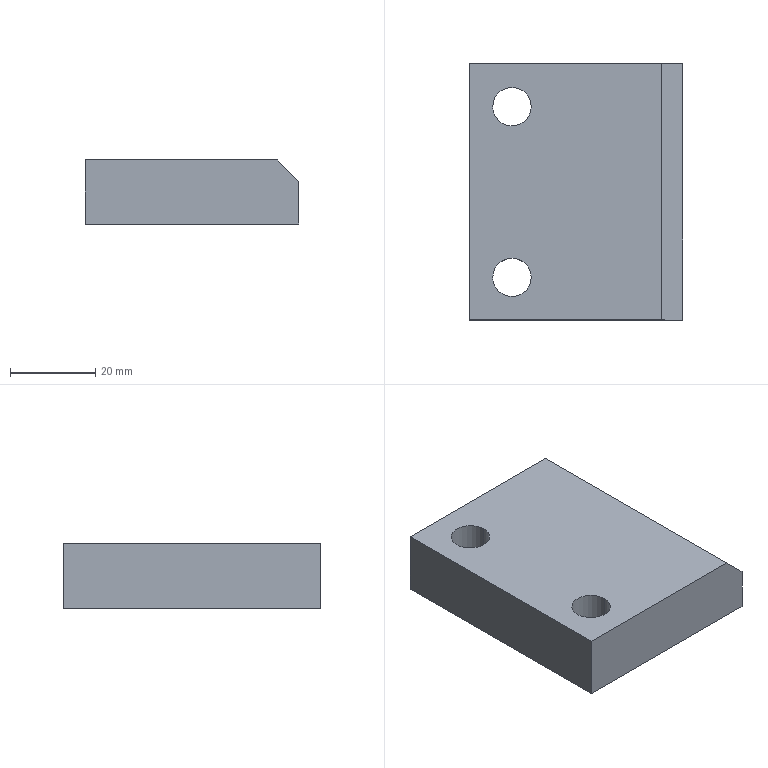Part | STEP file | Positioning_id1330_x_t | 1 solid | 11 faces | box 50 x 60 x 15 mm | volume 42341 mm3 | plane 7 | cylinder 4 | commonest cylinder face diameters 9 x4
STEP:
#1=CARTESIAN_POINT('',(0.,0.,0.));
#2=DIRECTION('',(0.,0.,1.));
#3=DIRECTION('',(1.,0.,0.));
#4=AXIS2_PLACEMENT_3D('',#1,#2,#3);
#5=CARTESIAN_POINT('',(-1027.502,770.,87.466));
#6=VERTEX_POINT('',#5);
#7=CARTESIAN_POINT('',(-1018.502,770.,87.466));
#8=VERTEX_POINT('',#7);
#9=CARTESIAN_POINT('',(-1023.002,770.,87.466));
#10=DIRECTION('',(0.,0.,-1.));
#11=DIRECTION('',(-1.,0.,0.));
#12=AXIS2_PLACEMENT_3D('',#9,#10,#11);
#13=CIRCLE('',#12,4.5);
#14=CARTESIAN_POINT('',(-1023.002,770.,72.466));
#15=DIRECTION('',(0.,0.,-1.));
#16=DIRECTION('',(-1.,0.,0.));
#17=AXIS2_PLACEMENT_3D('',#14,#15,#16);
#18=CYLINDRICAL_SURFACE('',#17,4.5);
#19=CARTESIAN_POINT('',(0.,-15.));
#20=DIRECTION('',(1.,0.));
#21=VECTOR('',#20,1.);
#22=LINE('',#19,#21);
#23=(GEOMETRIC_REPRESENTATION_CONTEXT(2)PARAMETRIC_REPRESENTATION_CONTEXT()REPRESENTATION_CONTEXT('',''));
#24=DEFINITIONAL_REPRESENTATION('',(#22),#23);
#25=PCURVE('',#18,#24);
#26=CARTESIAN_POINT('',(-1008.002,760.,87.466));
#27=DIRECTION('',(0.,0.,1.));
#28=DIRECTION('',(0.,1.,0.));
#29=AXIS2_PLACEMENT_3D('',#26,#27,#28);
#30=PLANE('',#29);
#31=CARTESIAN_POINT('',(10.,19.5));
#32=CARTESIAN_POINT('',(17.794,19.5));
#33=CARTESIAN_POINT('',(13.897,12.75));
#34=CARTESIAN_POINT('',(10.,6.));
#35=CARTESIAN_POINT('',(6.103,12.75));
#36=CARTESIAN_POINT('',(2.206,19.5));
#37=CARTESIAN_POINT('',(10.,19.5));
#38=(BOUNDED_CURVE()B_SPLINE_CURVE(2,(#31,#32,#33,#34,#35,#36,#37),.UNSPECIFIED.,.T.,.F.)B_SPLINE_CURVE_WITH_KNOTS((1,2,2,2,2,1),(-2.094,0.,2.094,4.189,6.283,8.378),.UNSPECIFIED.)CURVE()GEOMETRIC_REPRESENTATION_ITEM()RATIONAL_B_SPLINE_CURVE((1.,0.5,1.,0.5,1.,0.5,1.))REPRESENTATION_ITEM(''));
#39=(GEOMETRIC_REPRESENTATION_CONTEXT(2)PARAMETRIC_REPRESENTATION_CONTEXT()REPRESENTATION_CONTEXT('',''));
#40=DEFINITIONAL_REPRESENTATION('',(#38),#39);
#41=PCURVE('',#30,#40);
#42=SURFACE_CURVE('',#13,(#25,#41),.PCURVE_S1.);
#43=EDGE_CURVE('',#6,#8,#42,.T.);
#44=ORIENTED_EDGE('',*,*,#43,.T.);
#45=CARTESIAN_POINT('',(-1018.502,770.,72.466));
#46=VERTEX_POINT('',#45);
#47=CARTESIAN_POINT('',(-1018.502,770.,72.466));
#48=DIRECTION('',(0.,0.,-1.));
#49=VECTOR('',#48,1.);
#50=LINE('',#47,#49);
#51=CARTESIAN_POINT('',(3.142,0.));
#52=DIRECTION('',(0.,1.));
#53=VECTOR('',#52,1.);
#54=LINE('',#51,#53);
#55=(GEOMETRIC_REPRESENTATION_CONTEXT(2)PARAMETRIC_REPRESENTATION_CONTEXT()REPRESENTATION_CONTEXT('',''));
#56=DEFINITIONAL_REPRESENTATION('',(#54),#55);
#57=PCURVE('',#18,#56);
#58=CARTESIAN_POINT('',(-1023.002,770.,72.466));
#59=DIRECTION('',(0.,0.,-1.));
#60=DIRECTION('',(-1.,0.,0.));
#61=AXIS2_PLACEMENT_3D('',#58,#59,#60);
#62=CYLINDRICAL_SURFACE('',#61,4.5);
#63=CARTESIAN_POINT('',(3.142,0.));
#64=DIRECTION('',(0.,1.));
#65=VECTOR('',#64,1.);
#66=LINE('',#63,#65);
#67=(GEOMETRIC_REPRESENTATION_CONTEXT(2)PARAMETRIC_REPRESENTATION_CONTEXT()REPRESENTATION_CONTEXT('',''));
#68=DEFINITIONAL_REPRESENTATION('',(#66),#67);
#69=PCURVE('',#62,#68);
#70=SURFACE_CURVE('',#50,(#57,#69),.PCURVE_S1.);
#71=EDGE_CURVE('',#8,#46,#70,.T.);
#72=ORIENTED_EDGE('',*,*,#71,.T.);
#73=CARTESIAN_POINT('',(-1027.502,770.,72.466));
#74=VERTEX_POINT('',#73);
#75=CARTESIAN_POINT('',(-1023.002,770.,72.466));
#76=DIRECTION('',(0.,0.,-1.));
#77=DIRECTION('',(-1.,0.,0.));
#78=AXIS2_PLACEMENT_3D('',#75,#76,#77);
#79=CIRCLE('',#78,4.5);
#80=CARTESIAN_POINT('',(0.,0.));
#81=DIRECTION('',(1.,0.));
#82=VECTOR('',#81,1.);
#83=LINE('',#80,#82);
#84=(GEOMETRIC_REPRESENTATION_CONTEXT(2)PARAMETRIC_REPRESENTATION_CONTEXT()REPRESENTATION_CONTEXT('',''));
#85=DEFINITIONAL_REPRESENTATION('',(#83),#84);
#86=PCURVE('',#18,#85);
#87=CARTESIAN_POINT('',(-1008.002,760.,72.466));
#88=DIRECTION('',(0.,0.,-1.));
#89=DIRECTION('',(0.,-1.,0.));
#90=AXIS2_PLACEMENT_3D('',#87,#88,#89);
#91=PLANE('',#90);
#92=CARTESIAN_POINT('',(-10.,15.));
#93=DIRECTION('',(0.,1.));
#94=AXIS2_PLACEMENT_2D('',#92,#93);
#95=CIRCLE('',#94,4.5);
#96=(GEOMETRIC_REPRESENTATION_CONTEXT(2)PARAMETRIC_REPRESENTATION_CONTEXT()REPRESENTATION_CONTEXT('',''));
#97=DEFINITIONAL_REPRESENTATION('',(#95),#96);
#98=PCURVE('',#91,#97);
#99=SURFACE_CURVE('',#79,(#86,#98),.PCURVE_S1.);
#100=EDGE_CURVE('',#74,#46,#99,.T.);
#101=ORIENTED_EDGE('',*,*,#100,.F.);
#102=CARTESIAN_POINT('',(-1027.502,770.,72.466));
#103=DIRECTION('',(0.,0.,1.));
#104=VECTOR('',#103,1.);
#105=LINE('',#102,#104);
#106=CARTESIAN_POINT('',(0.,0.));
#107=DIRECTION('',(0.,-1.));
#108=VECTOR('',#107,1.);
#109=LINE('',#106,#108);
#110=(GEOMETRIC_REPRESENTATION_CONTEXT(2)PARAMETRIC_REPRESENTATION_CONTEXT()REPRESENTATION_CONTEXT('',''));
#111=DEFINITIONAL_REPRESENTATION('',(#109),#110);
#112=PCURVE('',#18,#111);
#113=CARTESIAN_POINT('',(6.283,0.));
#114=DIRECTION('',(0.,-1.));
#115=VECTOR('',#114,1.);
#116=LINE('',#113,#115);
#117=(GEOMETRIC_REPRESENTATION_CONTEXT(2)PARAMETRIC_REPRESENTATION_CONTEXT()REPRESENTATION_CONTEXT('',''));
#118=DEFINITIONAL_REPRESENTATION('',(#116),#117);
#119=PCURVE('',#62,#118);
#120=SURFACE_CURVE('',#105,(#112,#119),.PCURVE_S1.);
#121=EDGE_CURVE('',#74,#6,#120,.T.);
#122=ORIENTED_EDGE('',*,*,#121,.T.);
#123=EDGE_LOOP('',(#44,#72,#101,#122));
#124=FACE_BOUND('',#123,.F.);
#125=ADVANCED_FACE('',(#124),#18,.F.);
#126=CARTESIAN_POINT('',(-1027.502,810.,87.466));
#127=VERTEX_POINT('',#126);
#128=CARTESIAN_POINT('',(-1018.502,810.,87.466));
#129=VERTEX_POINT('',#128);
#130=CARTESIAN_POINT('',(-1023.002,810.,87.466));
#131=DIRECTION('',(0.,0.,-1.));
#132=DIRECTION('',(-1.,0.,0.));
#133=AXIS2_PLACEMENT_3D('',#130,#131,#132);
#134=CIRCLE('',#133,4.5);
#135=CARTESIAN_POINT('',(-1023.002,810.,72.466));
#136=DIRECTION('',(0.,0.,-1.));
#137=DIRECTION('',(-1.,0.,0.));
#138=AXIS2_PLACEMENT_3D('',#135,#136,#137);
#139=CYLINDRICAL_SURFACE('',#138,4.5);
#140=CARTESIAN_POINT('',(0.,-15.));
#141=DIRECTION('',(1.,0.));
#142=VECTOR('',#141,1.);
#143=LINE('',#140,#142);
#144=(GEOMETRIC_REPRESENTATION_CONTEXT(2)PARAMETRIC_REPRESENTATION_CONTEXT()REPRESENTATION_CONTEXT('',''));
#145=DEFINITIONAL_REPRESENTATION('',(#143),#144);
#146=PCURVE('',#139,#145);
#147=CARTESIAN_POINT('',(50.,19.5));
#148=CARTESIAN_POINT('',(57.794,19.5));
#149=CARTESIAN_POINT('',(53.897,12.75));
#150=CARTESIAN_POINT('',(50.,6.));
#151=CARTESIAN_POINT('',(46.103,12.75));
#152=CARTESIAN_POINT('',(42.206,19.5));
#153=CARTESIAN_POINT('',(50.,19.5));
#154=(BOUNDED_CURVE()B_SPLINE_CURVE(2,(#147,#148,#149,#150,#151,#152,#153),.UNSPECIFIED.,.T.,.F.)B_SPLINE_CURVE_WITH_KNOTS((1,2,2,2,2,1),(-2.094,0.,2.094,4.189,6.283,8.378),.UNSPECIFIED.)CURVE()GEOMETRIC_REPRESENTATION_ITEM()RATIONAL_B_SPLINE_CURVE((1.,0.5,1.,0.5,1.,0.5,1.))REPRESENTATION_ITEM(''));
#155=(GEOMETRIC_REPRESENTATION_CONTEXT(2)PARAMETRIC_REPRESENTATION_CONTEXT()REPRESENTATION_CONTEXT('',''));
#156=DEFINITIONAL_REPRESENTATION('',(#154),#155);
#157=PCURVE('',#30,#156);
#158=SURFACE_CURVE('',#134,(#146,#157),.PCURVE_S1.);
#159=EDGE_CURVE('',#127,#129,#158,.T.);
#160=ORIENTED_EDGE('',*,*,#159,.T.);
#161=CARTESIAN_POINT('',(-1018.502,810.,72.466));
#162=VERTEX_POINT('',#161);
#163=CARTESIAN_POINT('',(-1018.502,810.,72.466));
#164=DIRECTION('',(0.,0.,-1.));
#165=VECTOR('',#164,1.);
#166=LINE('',#163,#165);
#167=CARTESIAN_POINT('',(3.142,0.));
#168=DIRECTION('',(0.,1.));
#169=VECTOR('',#168,1.);
#170=LINE('',#167,#169);
#171=(GEOMETRIC_REPRESENTATION_CONTEXT(2)PARAMETRIC_REPRESENTATION_CONTEXT()REPRESENTATION_CONTEXT('',''));
#172=DEFINITIONAL_REPRESENTATION('',(#170),#171);
#173=PCURVE('',#139,#172);
#174=CARTESIAN_POINT('',(-1023.002,810.,72.466));
#175=DIRECTION('',(0.,0.,-1.));
#176=DIRECTION('',(-1.,0.,0.));
#177=AXIS2_PLACEMENT_3D('',#174,#175,#176);
#178=CYLINDRICAL_SURFACE('',#177,4.5);
#179=CARTESIAN_POINT('',(3.142,0.));
#180=DIRECTION('',(0.,1.));
#181=VECTOR('',#180,1.);
#182=LINE('',#179,#181);
#183=(GEOMETRIC_REPRESENTATION_CONTEXT(2)PARAMETRIC_REPRESENTATION_CONTEXT()REPRESENTATION_CONTEXT('',''));
#184=DEFINITIONAL_REPRESENTATION('',(#182),#183);
#185=PCURVE('',#178,#184);
#186=SURFACE_CURVE('',#166,(#173,#185),.PCURVE_S1.);
#187=EDGE_CURVE('',#129,#162,#186,.T.);
#188=ORIENTED_EDGE('',*,*,#187,.T.);
#189=CARTESIAN_POINT('',(-1027.502,810.,72.466));
#190=VERTEX_POINT('',#189);
#191=CARTESIAN_POINT('',(-1023.002,810.,72.466));
#192=DIRECTION('',(0.,0.,-1.));
#193=DIRECTION('',(-1.,0.,0.));
#194=AXIS2_PLACEMENT_3D('',#191,#192,#193);
#195=CIRCLE('',#194,4.5);
#196=CARTESIAN_POINT('',(0.,0.));
#197=DIRECTION('',(1.,0.));
#198=VECTOR('',#197,1.);
#199=LINE('',#196,#198);
#200=(GEOMETRIC_REPRESENTATION_CONTEXT(2)PARAMETRIC_REPRESENTATION_CONTEXT()REPRESENTATION_CONTEXT('',''));
#201=DEFINITIONAL_REPRESENTATION('',(#199),#200);
#202=PCURVE('',#139,#201);
#203=CARTESIAN_POINT('',(-50.,15.));
#204=DIRECTION('',(0.,1.));
#205=AXIS2_PLACEMENT_2D('',#203,#204);
#206=CIRCLE('',#205,4.5);
#207=(GEOMETRIC_REPRESENTATION_CONTEXT(2)PARAMETRIC_REPRESENTATION_CONTEXT()REPRESENTATION_CONTEXT('',''));
#208=DEFINITIONAL_REPRESENTATION('',(#206),#207);
#209=PCURVE('',#91,#208);
#210=SURFACE_CURVE('',#195,(#202,#209),.PCURVE_S1.);
#211=EDGE_CURVE('',#190,#162,#210,.T.);
#212=ORIENTED_EDGE('',*,*,#211,.F.);
#213=CARTESIAN_POINT('',(-1027.502,810.,72.466));
#214=DIRECTION('',(0.,0.,1.));
#215=VECTOR('',#214,1.);
#216=LINE('',#213,#215);
#217=CARTESIAN_POINT('',(0.,0.));
#218=DIRECTION('',(0.,-1.));
#219=VECTOR('',#218,1.);
#220=LINE('',#217,#219);
#221=(GEOMETRIC_REPRESENTATION_CONTEXT(2)PARAMETRIC_REPRESENTATION_CONTEXT()REPRESENTATION_CONTEXT('',''));
#222=DEFINITIONAL_REPRESENTATION('',(#220),#221);
#223=PCURVE('',#139,#222);
#224=CARTESIAN_POINT('',(6.283,0.));
#225=DIRECTION('',(0.,-1.));
#226=VECTOR('',#225,1.);
#227=LINE('',#224,#226);
#228=(GEOMETRIC_REPRESENTATION_CONTEXT(2)PARAMETRIC_REPRESENTATION_CONTEXT()REPRESENTATION_CONTEXT('',''));
#229=DEFINITIONAL_REPRESENTATION('',(#227),#228);
#230=PCURVE('',#178,#229);
#231=SURFACE_CURVE('',#216,(#223,#230),.PCURVE_S1.);
#232=EDGE_CURVE('',#190,#127,#231,.T.);
#233=ORIENTED_EDGE('',*,*,#232,.T.);
#234=EDGE_LOOP('',(#160,#188,#212,#233));
#235=FACE_BOUND('',#234,.F.);
#236=ADVANCED_FACE('',(#235),#139,.F.);
#237=CARTESIAN_POINT('',(-988.002,760.,87.466));
#238=VERTEX_POINT('',#237);
#239=CARTESIAN_POINT('',(-983.002,760.,82.466));
#240=VERTEX_POINT('',#239);
#241=CARTESIAN_POINT('',(-988.002,760.,87.466));
#242=DIRECTION('',(0.7071,0.,-0.7071));
#243=VECTOR('',#242,1.);
#244=LINE('',#241,#243);
#245=CARTESIAN_POINT('',(-983.002,760.,82.466));
#246=DIRECTION('',(-0.7071,0.,-0.7071));
#247=DIRECTION('',(0.7071,0.,-0.7071));
#248=AXIS2_PLACEMENT_3D('',#245,#246,#247);
#249=PLANE('',#248);
#250=CARTESIAN_POINT('',(-7.071,0.));
#251=DIRECTION('',(1.,0.));
#252=VECTOR('',#251,1.);
#253=LINE('',#250,#252);
#254=(GEOMETRIC_REPRESENTATION_CONTEXT(2)PARAMETRIC_REPRESENTATION_CONTEXT()REPRESENTATION_CONTEXT('',''));
#255=DEFINITIONAL_REPRESENTATION('',(#253),#254);
#256=PCURVE('',#249,#255);
#257=CARTESIAN_POINT('',(-1008.002,760.,79.966));
#258=DIRECTION('',(0.,-1.,0.));
#259=DIRECTION('',(0.,0.,1.));
#260=AXIS2_PLACEMENT_3D('',#257,#258,#259);
#261=PLANE('',#260);
#262=CARTESIAN_POINT('',(7.5,-20.));
#263=DIRECTION('',(-0.7071,-0.7071));
#264=VECTOR('',#263,1.);
#265=LINE('',#262,#264);
#266=(GEOMETRIC_REPRESENTATION_CONTEXT(2)PARAMETRIC_REPRESENTATION_CONTEXT()REPRESENTATION_CONTEXT('',''));
#267=DEFINITIONAL_REPRESENTATION('',(#265),#266);
#268=PCURVE('',#261,#267);
#269=SURFACE_CURVE('',#244,(#256,#268),.PCURVE_S1.);
#270=EDGE_CURVE('',#238,#240,#269,.T.);
#271=ORIENTED_EDGE('',*,*,#270,.T.);
#272=CARTESIAN_POINT('',(-983.002,820.,82.466));
#273=VERTEX_POINT('',#272);
#274=CARTESIAN_POINT('',(-983.002,760.,82.466));
#275=DIRECTION('',(0.,1.,0.));
#276=VECTOR('',#275,1.);
#277=LINE('',#274,#276);
#278=CARTESIAN_POINT('',(0.,0.));
#279=DIRECTION('',(0.,-1.));
#280=VECTOR('',#279,1.);
#281=LINE('',#278,#280);
#282=(GEOMETRIC_REPRESENTATION_CONTEXT(2)PARAMETRIC_REPRESENTATION_CONTEXT()REPRESENTATION_CONTEXT('',''));
#283=DEFINITIONAL_REPRESENTATION('',(#281),#282);
#284=PCURVE('',#249,#283);
#285=CARTESIAN_POINT('',(-983.002,760.,79.966));
#286=DIRECTION('',(1.,0.,0.));
#287=DIRECTION('',(0.,1.,0.));
#288=AXIS2_PLACEMENT_3D('',#285,#286,#287);
#289=PLANE('',#288);
#290=CARTESIAN_POINT('',(0.,2.5));
#291=DIRECTION('',(1.,0.));
#292=VECTOR('',#291,1.);
#293=LINE('',#290,#292);
#294=(GEOMETRIC_REPRESENTATION_CONTEXT(2)PARAMETRIC_REPRESENTATION_CONTEXT()REPRESENTATION_CONTEXT('',''));
#295=DEFINITIONAL_REPRESENTATION('',(#293),#294);
#296=PCURVE('',#289,#295);
#297=SURFACE_CURVE('',#277,(#284,#296),.PCURVE_S1.);
#298=EDGE_CURVE('',#240,#273,#297,.T.);
#299=ORIENTED_EDGE('',*,*,#298,.T.);
#300=CARTESIAN_POINT('',(-988.002,820.,87.466));
#301=VERTEX_POINT('',#300);
#302=CARTESIAN_POINT('',(-983.002,820.,82.466));
#303=DIRECTION('',(-0.7071,0.,0.7071));
#304=VECTOR('',#303,1.);
#305=LINE('',#302,#304);
#306=CARTESIAN_POINT('',(0.,-60.));
#307=DIRECTION('',(-1.,0.));
#308=VECTOR('',#307,1.);
#309=LINE('',#306,#308);
#310=(GEOMETRIC_REPRESENTATION_CONTEXT(2)PARAMETRIC_REPRESENTATION_CONTEXT()REPRESENTATION_CONTEXT('',''));
#311=DEFINITIONAL_REPRESENTATION('',(#309),#310);
#312=PCURVE('',#249,#311);
#313=CARTESIAN_POINT('',(-1008.002,820.,79.966));
#314=DIRECTION('',(0.,1.,0.));
#315=DIRECTION('',(0.,0.,-1.));
#316=AXIS2_PLACEMENT_3D('',#313,#314,#315);
#317=PLANE('',#316);
#318=CARTESIAN_POINT('',(-2.5,-25.));
#319=DIRECTION('',(-0.7071,0.7071));
#320=VECTOR('',#319,1.);
#321=LINE('',#318,#320);
#322=(GEOMETRIC_REPRESENTATION_CONTEXT(2)PARAMETRIC_REPRESENTATION_CONTEXT()REPRESENTATION_CONTEXT('',''));
#323=DEFINITIONAL_REPRESENTATION('',(#321),#322);
#324=PCURVE('',#317,#323);
#325=SURFACE_CURVE('',#305,(#312,#324),.PCURVE_S1.);
#326=EDGE_CURVE('',#273,#301,#325,.T.);
#327=ORIENTED_EDGE('',*,*,#326,.T.);
#328=CARTESIAN_POINT('',(-988.002,820.,87.466));
#329=DIRECTION('',(0.,-1.,0.));
#330=VECTOR('',#329,1.);
#331=LINE('',#328,#330);
#332=CARTESIAN_POINT('',(-7.071,-60.));
#333=DIRECTION('',(0.,1.));
#334=VECTOR('',#333,1.);
#335=LINE('',#332,#334);
#336=(GEOMETRIC_REPRESENTATION_CONTEXT(2)PARAMETRIC_REPRESENTATION_CONTEXT()REPRESENTATION_CONTEXT('',''));
#337=DEFINITIONAL_REPRESENTATION('',(#335),#336);
#338=PCURVE('',#249,#337);
#339=CARTESIAN_POINT('',(60.,-20.));
#340=DIRECTION('',(-1.,0.));
#341=VECTOR('',#340,1.);
#342=LINE('',#339,#341);
#343=(GEOMETRIC_REPRESENTATION_CONTEXT(2)PARAMETRIC_REPRESENTATION_CONTEXT()REPRESENTATION_CONTEXT('',''));
#344=DEFINITIONAL_REPRESENTATION('',(#342),#343);
#345=PCURVE('',#30,#344);
#346=SURFACE_CURVE('',#331,(#338,#345),.PCURVE_S1.);
#347=EDGE_CURVE('',#301,#238,#346,.T.);
#348=ORIENTED_EDGE('',*,*,#347,.T.);
#349=EDGE_LOOP('',(#271,#299,#327,#348));
#350=FACE_BOUND('',#349,.T.);
#351=ADVANCED_FACE('',(#350),#249,.F.);
#352=CARTESIAN_POINT('',(-1018.502,810.,87.466));
#353=CARTESIAN_POINT('',(-1018.502,805.5,87.466));
#354=CARTESIAN_POINT('',(-1023.002,803.25,87.466));
#355=CARTESIAN_POINT('',(-1027.502,805.5,87.466));
#356=CARTESIAN_POINT('',(-1027.502,810.,87.466));
#357=(BOUNDED_CURVE()B_SPLINE_CURVE(4,(#352,#353,#354,#355,#356),.UNSPECIFIED.,.F.,.F.)B_SPLINE_CURVE_WITH_KNOTS((5,5),(0.,1.),.PIECEWISE_BEZIER_KNOTS.)CURVE()GEOMETRIC_REPRESENTATION_ITEM()RATIONAL_B_SPLINE_CURVE((1.,0.7071,0.6667,0.7071,1.))REPRESENTATION_ITEM(''));
#358=CARTESIAN_POINT('',(50.,10.5));
#359=CARTESIAN_POINT('',(45.5,10.5));
#360=CARTESIAN_POINT('',(43.25,15.));
#361=CARTESIAN_POINT('',(45.5,19.5));
#362=CARTESIAN_POINT('',(50.,19.5));
#363=(BOUNDED_CURVE()B_SPLINE_CURVE(4,(#358,#359,#360,#361,#362),.UNSPECIFIED.,.F.,.F.)B_SPLINE_CURVE_WITH_KNOTS((5,5),(0.,1.),.PIECEWISE_BEZIER_KNOTS.)CURVE()GEOMETRIC_REPRESENTATION_ITEM()RATIONAL_B_SPLINE_CURVE((1.,0.7071,0.6667,0.7071,1.))REPRESENTATION_ITEM(''));
#364=(GEOMETRIC_REPRESENTATION_CONTEXT(2)PARAMETRIC_REPRESENTATION_CONTEXT()REPRESENTATION_CONTEXT('',''));
#365=DEFINITIONAL_REPRESENTATION('',(#363),#364);
#366=PCURVE('',#30,#365);
#367=CARTESIAN_POINT('',(3.142,-15.));
#368=CARTESIAN_POINT('',(3.184,-15.));
#369=CARTESIAN_POINT('',(3.271,-15.));
#370=CARTESIAN_POINT('',(3.405,-15.));
#371=CARTESIAN_POINT('',(3.542,-15.));
#372=CARTESIAN_POINT('',(3.681,-15.));
#373=CARTESIAN_POINT('',(3.823,-15.));
#374=CARTESIAN_POINT('',(3.968,-15.));
#375=CARTESIAN_POINT('',(4.114,-15.));
#376=CARTESIAN_POINT('',(4.262,-15.));
#377=CARTESIAN_POINT('',(4.412,-15.));
#378=CARTESIAN_POINT('',(4.562,-15.));
#379=CARTESIAN_POINT('',(4.712,-15.));
#380=CARTESIAN_POINT('',(4.863,-15.));
#381=CARTESIAN_POINT('',(5.013,-15.));
#382=CARTESIAN_POINT('',(5.163,-15.));
#383=CARTESIAN_POINT('',(5.311,-15.));
#384=CARTESIAN_POINT('',(5.457,-15.));
#385=CARTESIAN_POINT('',(5.602,-15.));
#386=CARTESIAN_POINT('',(5.744,-15.));
#387=CARTESIAN_POINT('',(5.883,-15.));
#388=CARTESIAN_POINT('',(6.02,-15.));
#389=CARTESIAN_POINT('',(6.153,-15.));
#390=CARTESIAN_POINT('',(6.24,-15.));
#391=CARTESIAN_POINT('',(6.283,-15.));
#392=B_SPLINE_CURVE_WITH_KNOTS('',3,(#367,#368,#369,#370,#371,#372,#373,#374,#375,#376,#377,#378,#379,#380,#381,#382,#383,#384,#385,#386,#387,#388,#389,#390,#391),.UNSPECIFIED.,.F.,.F.,(4,1,1,1,1,1,1,1,1,1,1,1,1,1,1,1,1,1,1,1,1,1,4),(0.,0.04545,0.09091,0.1364,0.1818,0.2273,0.2727,0.3182,0.3636,0.4091,0.4545,0.5,0.5455,0.5909,0.6364,0.6818,0.7273,0.7727,0.8182,0.8636,0.9091,0.9545,1.),.QUASI_UNIFORM_KNOTS.);
#393=(GEOMETRIC_REPRESENTATION_CONTEXT(2)PARAMETRIC_REPRESENTATION_CONTEXT()REPRESENTATION_CONTEXT('',''));
#394=DEFINITIONAL_REPRESENTATION('',(#392),#393);
#395=PCURVE('',#178,#394);
#396=SURFACE_CURVE('',#357,(#366,#395),.PCURVE_S1.);
#397=EDGE_CURVE('',#129,#127,#396,.T.);
#398=ORIENTED_EDGE('',*,*,#397,.T.);
#399=ORIENTED_EDGE('',*,*,#159,.T.);
#400=EDGE_LOOP('',(#398,#399));
#401=FACE_BOUND('',#400,.T.);
#402=CARTESIAN_POINT('',(-1018.502,770.,87.466));
#403=CARTESIAN_POINT('',(-1018.502,765.5,87.466));
#404=CARTESIAN_POINT('',(-1023.002,763.25,87.466));
#405=CARTESIAN_POINT('',(-1027.502,765.5,87.466));
#406=CARTESIAN_POINT('',(-1027.502,770.,87.466));
#407=(BOUNDED_CURVE()B_SPLINE_CURVE(4,(#402,#403,#404,#405,#406),.UNSPECIFIED.,.F.,.F.)B_SPLINE_CURVE_WITH_KNOTS((5,5),(0.,1.),.PIECEWISE_BEZIER_KNOTS.)CURVE()GEOMETRIC_REPRESENTATION_ITEM()RATIONAL_B_SPLINE_CURVE((1.,0.7071,0.6667,0.7071,1.))REPRESENTATION_ITEM(''));
#408=CARTESIAN_POINT('',(10.,10.5));
#409=CARTESIAN_POINT('',(5.5,10.5));
#410=CARTESIAN_POINT('',(3.25,15.));
#411=CARTESIAN_POINT('',(5.5,19.5));
#412=CARTESIAN_POINT('',(10.,19.5));
#413=(BOUNDED_CURVE()B_SPLINE_CURVE(4,(#408,#409,#410,#411,#412),.UNSPECIFIED.,.F.,.F.)B_SPLINE_CURVE_WITH_KNOTS((5,5),(0.,1.),.PIECEWISE_BEZIER_KNOTS.)CURVE()GEOMETRIC_REPRESENTATION_ITEM()RATIONAL_B_SPLINE_CURVE((1.,0.7071,0.6667,0.7071,1.))REPRESENTATION_ITEM(''));
#414=(GEOMETRIC_REPRESENTATION_CONTEXT(2)PARAMETRIC_REPRESENTATION_CONTEXT()REPRESENTATION_CONTEXT('',''));
#415=DEFINITIONAL_REPRESENTATION('',(#413),#414);
#416=PCURVE('',#30,#415);
#417=CARTESIAN_POINT('',(3.142,-15.));
#418=CARTESIAN_POINT('',(3.184,-15.));
#419=CARTESIAN_POINT('',(3.271,-15.));
#420=CARTESIAN_POINT('',(3.405,-15.));
#421=CARTESIAN_POINT('',(3.542,-15.));
#422=CARTESIAN_POINT('',(3.681,-15.));
#423=CARTESIAN_POINT('',(3.823,-15.));
#424=CARTESIAN_POINT('',(3.968,-15.));
#425=CARTESIAN_POINT('',(4.114,-15.));
#426=CARTESIAN_POINT('',(4.262,-15.));
#427=CARTESIAN_POINT('',(4.412,-15.));
#428=CARTESIAN_POINT('',(4.562,-15.));
#429=CARTESIAN_POINT('',(4.712,-15.));
#430=CARTESIAN_POINT('',(4.863,-15.));
#431=CARTESIAN_POINT('',(5.013,-15.));
#432=CARTESIAN_POINT('',(5.163,-15.));
#433=CARTESIAN_POINT('',(5.311,-15.));
#434=CARTESIAN_POINT('',(5.457,-15.));
#435=CARTESIAN_POINT('',(5.602,-15.));
#436=CARTESIAN_POINT('',(5.744,-15.));
#437=CARTESIAN_POINT('',(5.883,-15.));
#438=CARTESIAN_POINT('',(6.02,-15.));
#439=CARTESIAN_POINT('',(6.153,-15.));
#440=CARTESIAN_POINT('',(6.24,-15.));
#441=CARTESIAN_POINT('',(6.283,-15.));
#442=B_SPLINE_CURVE_WITH_KNOTS('',3,(#417,#418,#419,#420,#421,#422,#423,#424,#425,#426,#427,#428,#429,#430,#431,#432,#433,#434,#435,#436,#437,#438,#439,#440,#441),.UNSPECIFIED.,.F.,.F.,(4,1,1,1,1,1,1,1,1,1,1,1,1,1,1,1,1,1,1,1,1,1,4),(0.,0.04545,0.09091,0.1364,0.1818,0.2273,0.2727,0.3182,0.3636,0.4091,0.4545,0.5,0.5455,0.5909,0.6364,0.6818,0.7273,0.7727,0.8182,0.8636,0.9091,0.9545,1.),.QUASI_UNIFORM_KNOTS.);
#443=(GEOMETRIC_REPRESENTATION_CONTEXT(2)PARAMETRIC_REPRESENTATION_CONTEXT()REPRESENTATION_CONTEXT('',''));
#444=DEFINITIONAL_REPRESENTATION('',(#442),#443);
#445=PCURVE('',#62,#444);
#446=SURFACE_CURVE('',#407,(#416,#445),.PCURVE_S1.);
#447=EDGE_CURVE('',#8,#6,#446,.T.);
#448=ORIENTED_EDGE('',*,*,#447,.T.);
#449=ORIENTED_EDGE('',*,*,#43,.T.);
#450=EDGE_LOOP('',(#448,#449));
#451=FACE_BOUND('',#450,.T.);
#452=CARTESIAN_POINT('',(-1033.002,820.,87.466));
#453=VERTEX_POINT('',#452);
#454=CARTESIAN_POINT('',(-1033.002,820.,87.466));
#455=DIRECTION('',(1.,0.,0.));
#456=VECTOR('',#455,1.);
#457=LINE('',#454,#456);
#458=CARTESIAN_POINT('',(60.,25.));
#459=DIRECTION('',(0.,-1.));
#460=VECTOR('',#459,1.);
#461=LINE('',#458,#460);
#462=(GEOMETRIC_REPRESENTATION_CONTEXT(2)PARAMETRIC_REPRESENTATION_CONTEXT()REPRESENTATION_CONTEXT('',''));
#463=DEFINITIONAL_REPRESENTATION('',(#461),#462);
#464=PCURVE('',#30,#463);
#465=CARTESIAN_POINT('',(-7.5,25.));
#466=DIRECTION('',(0.,-1.));
#467=VECTOR('',#466,1.);
#468=LINE('',#465,#467);
#469=(GEOMETRIC_REPRESENTATION_CONTEXT(2)PARAMETRIC_REPRESENTATION_CONTEXT()REPRESENTATION_CONTEXT('',''));
#470=DEFINITIONAL_REPRESENTATION('',(#468),#469);
#471=PCURVE('',#317,#470);
#472=SURFACE_CURVE('',#457,(#464,#471),.PCURVE_S1.);
#473=EDGE_CURVE('',#453,#301,#472,.T.);
#474=ORIENTED_EDGE('',*,*,#473,.F.);
#475=CARTESIAN_POINT('',(-1033.002,760.,87.466));
#476=VERTEX_POINT('',#475);
#477=CARTESIAN_POINT('',(-1033.002,760.,87.466));
#478=DIRECTION('',(0.,1.,0.));
#479=VECTOR('',#478,1.);
#480=LINE('',#477,#479);
#481=CARTESIAN_POINT('',(0.,25.));
#482=DIRECTION('',(1.,0.));
#483=VECTOR('',#482,1.);
#484=LINE('',#481,#483);
#485=(GEOMETRIC_REPRESENTATION_CONTEXT(2)PARAMETRIC_REPRESENTATION_CONTEXT()REPRESENTATION_CONTEXT('',''));
#486=DEFINITIONAL_REPRESENTATION('',(#484),#485);
#487=PCURVE('',#30,#486);
#488=CARTESIAN_POINT('',(-1033.002,760.,79.966));
#489=DIRECTION('',(-1.,0.,0.));
#490=DIRECTION('',(0.,-1.,0.));
#491=AXIS2_PLACEMENT_3D('',#488,#489,#490);
#492=PLANE('',#491);
#493=CARTESIAN_POINT('',(0.,7.5));
#494=DIRECTION('',(-1.,0.));
#495=VECTOR('',#494,1.);
#496=LINE('',#493,#495);
#497=(GEOMETRIC_REPRESENTATION_CONTEXT(2)PARAMETRIC_REPRESENTATION_CONTEXT()REPRESENTATION_CONTEXT('',''));
#498=DEFINITIONAL_REPRESENTATION('',(#496),#497);
#499=PCURVE('',#492,#498);
#500=SURFACE_CURVE('',#480,(#487,#499),.PCURVE_S1.);
#501=EDGE_CURVE('',#476,#453,#500,.T.);
#502=ORIENTED_EDGE('',*,*,#501,.F.);
#503=CARTESIAN_POINT('',(-988.002,760.,87.466));
#504=DIRECTION('',(-1.,0.,0.));
#505=VECTOR('',#504,1.);
#506=LINE('',#503,#505);
#507=CARTESIAN_POINT('',(0.,-20.));
#508=DIRECTION('',(0.,1.));
#509=VECTOR('',#508,1.);
#510=LINE('',#507,#509);
#511=(GEOMETRIC_REPRESENTATION_CONTEXT(2)PARAMETRIC_REPRESENTATION_CONTEXT()REPRESENTATION_CONTEXT('',''));
#512=DEFINITIONAL_REPRESENTATION('',(#510),#511);
#513=PCURVE('',#30,#512);
#514=CARTESIAN_POINT('',(7.5,-20.));
#515=DIRECTION('',(0.,1.));
#516=VECTOR('',#515,1.);
#517=LINE('',#514,#516);
#518=(GEOMETRIC_REPRESENTATION_CONTEXT(2)PARAMETRIC_REPRESENTATION_CONTEXT()REPRESENTATION_CONTEXT('',''));
#519=DEFINITIONAL_REPRESENTATION('',(#517),#518);
#520=PCURVE('',#261,#519);
#521=SURFACE_CURVE('',#506,(#513,#520),.PCURVE_S1.);
#522=EDGE_CURVE('',#238,#476,#521,.T.);
#523=ORIENTED_EDGE('',*,*,#522,.F.);
#524=ORIENTED_EDGE('',*,*,#347,.F.);
#525=EDGE_LOOP('',(#474,#502,#523,#524));
#526=FACE_BOUND('',#525,.T.);
#527=ADVANCED_FACE('',(#401,#451,#526),#30,.T.);
#528=ORIENTED_EDGE('',*,*,#522,.T.);
#529=CARTESIAN_POINT('',(-1033.002,760.,72.466));
#530=VERTEX_POINT('',#529);
#531=CARTESIAN_POINT('',(-1033.002,760.,87.466));
#532=DIRECTION('',(0.,0.,-1.));
#533=VECTOR('',#532,1.);
#534=LINE('',#531,#533);
#535=CARTESIAN_POINT('',(7.5,25.));
#536=DIRECTION('',(-1.,0.));
#537=VECTOR('',#536,1.);
#538=LINE('',#535,#537);
#539=(GEOMETRIC_REPRESENTATION_CONTEXT(2)PARAMETRIC_REPRESENTATION_CONTEXT()REPRESENTATION_CONTEXT('',''));
#540=DEFINITIONAL_REPRESENTATION('',(#538),#539);
#541=PCURVE('',#261,#540);
#542=CARTESIAN_POINT('',(0.,7.5));
#543=DIRECTION('',(0.,-1.));
#544=VECTOR('',#543,1.);
#545=LINE('',#542,#544);
#546=(GEOMETRIC_REPRESENTATION_CONTEXT(2)PARAMETRIC_REPRESENTATION_CONTEXT()REPRESENTATION_CONTEXT('',''));
#547=DEFINITIONAL_REPRESENTATION('',(#545),#546);
#548=PCURVE('',#492,#547);
#549=SURFACE_CURVE('',#534,(#541,#548),.PCURVE_S1.);
#550=EDGE_CURVE('',#476,#530,#549,.T.);
#551=ORIENTED_EDGE('',*,*,#550,.T.);
#552=CARTESIAN_POINT('',(-983.002,760.,72.466));
#553=VERTEX_POINT('',#552);
#554=CARTESIAN_POINT('',(-1033.002,760.,72.466));
#555=DIRECTION('',(1.,0.,0.));
#556=VECTOR('',#555,1.);
#557=LINE('',#554,#556);
#558=CARTESIAN_POINT('',(-7.5,25.));
#559=DIRECTION('',(0.,-1.));
#560=VECTOR('',#559,1.);
#561=LINE('',#558,#560);
#562=(GEOMETRIC_REPRESENTATION_CONTEXT(2)PARAMETRIC_REPRESENTATION_CONTEXT()REPRESENTATION_CONTEXT('',''));
#563=DEFINITIONAL_REPRESENTATION('',(#561),#562);
#564=PCURVE('',#261,#563);
#565=CARTESIAN_POINT('',(0.,25.));
#566=DIRECTION('',(0.,-1.));
#567=VECTOR('',#566,1.);
#568=LINE('',#565,#567);
#569=(GEOMETRIC_REPRESENTATION_CONTEXT(2)PARAMETRIC_REPRESENTATION_CONTEXT()REPRESENTATION_CONTEXT('',''));
#570=DEFINITIONAL_REPRESENTATION('',(#568),#569);
#571=PCURVE('',#91,#570);
#572=SURFACE_CURVE('',#557,(#564,#571),.PCURVE_S1.);
#573=EDGE_CURVE('',#530,#553,#572,.T.);
#574=ORIENTED_EDGE('',*,*,#573,.T.);
#575=CARTESIAN_POINT('',(-983.002,760.,72.466));
#576=DIRECTION('',(0.,0.,1.));
#577=VECTOR('',#576,1.);
#578=LINE('',#575,#577);
#579=CARTESIAN_POINT('',(-7.5,-25.));
#580=DIRECTION('',(1.,0.));
#581=VECTOR('',#580,1.);
#582=LINE('',#579,#581);
#583=(GEOMETRIC_REPRESENTATION_CONTEXT(2)PARAMETRIC_REPRESENTATION_CONTEXT()REPRESENTATION_CONTEXT('',''));
#584=DEFINITIONAL_REPRESENTATION('',(#582),#583);
#585=PCURVE('',#261,#584);
#586=CARTESIAN_POINT('',(0.,-7.5));
#587=DIRECTION('',(0.,1.));
#588=VECTOR('',#587,1.);
#589=LINE('',#586,#588);
#590=(GEOMETRIC_REPRESENTATION_CONTEXT(2)PARAMETRIC_REPRESENTATION_CONTEXT()REPRESENTATION_CONTEXT('',''));
#591=DEFINITIONAL_REPRESENTATION('',(#589),#590);
#592=PCURVE('',#289,#591);
#593=SURFACE_CURVE('',#578,(#585,#592),.PCURVE_S1.);
#594=EDGE_CURVE('',#553,#240,#593,.T.);
#595=ORIENTED_EDGE('',*,*,#594,.T.);
#596=ORIENTED_EDGE('',*,*,#270,.F.);
#597=EDGE_LOOP('',(#528,#551,#574,#595,#596));
#598=FACE_BOUND('',#597,.T.);
#599=ADVANCED_FACE('',(#598),#261,.T.);
#600=CARTESIAN_POINT('',(-1033.002,820.,72.466));
#601=VERTEX_POINT('',#600);
#602=CARTESIAN_POINT('',(-1033.002,760.,72.466));
#603=DIRECTION('',(0.,1.,0.));
#604=VECTOR('',#603,1.);
#605=LINE('',#602,#604);
#606=CARTESIAN_POINT('',(0.,-7.5));
#607=DIRECTION('',(-1.,0.));
#608=VECTOR('',#607,1.);
#609=LINE('',#606,#608);
#610=(GEOMETRIC_REPRESENTATION_CONTEXT(2)PARAMETRIC_REPRESENTATION_CONTEXT()REPRESENTATION_CONTEXT('',''));
#611=DEFINITIONAL_REPRESENTATION('',(#609),#610);
#612=PCURVE('',#492,#611);
#613=CARTESIAN_POINT('',(0.,25.));
#614=DIRECTION('',(-1.,0.));
#615=VECTOR('',#614,1.);
#616=LINE('',#613,#615);
#617=(GEOMETRIC_REPRESENTATION_CONTEXT(2)PARAMETRIC_REPRESENTATION_CONTEXT()REPRESENTATION_CONTEXT('',''));
#618=DEFINITIONAL_REPRESENTATION('',(#616),#617);
#619=PCURVE('',#91,#618);
#620=SURFACE_CURVE('',#605,(#612,#619),.PCURVE_S1.);
#621=EDGE_CURVE('',#530,#601,#620,.T.);
#622=ORIENTED_EDGE('',*,*,#621,.F.);
#623=ORIENTED_EDGE('',*,*,#550,.F.);
#624=ORIENTED_EDGE('',*,*,#501,.T.);
#625=CARTESIAN_POINT('',(-1033.002,820.,72.466));
#626=DIRECTION('',(0.,0.,1.));
#627=VECTOR('',#626,1.);
#628=LINE('',#625,#627);
#629=CARTESIAN_POINT('',(-60.,-7.5));
#630=DIRECTION('',(0.,1.));
#631=VECTOR('',#630,1.);
#632=LINE('',#629,#631);
#633=(GEOMETRIC_REPRESENTATION_CONTEXT(2)PARAMETRIC_REPRESENTATION_CONTEXT()REPRESENTATION_CONTEXT('',''));
#634=DEFINITIONAL_REPRESENTATION('',(#632),#633);
#635=PCURVE('',#492,#634);
#636=CARTESIAN_POINT('',(7.5,25.));
#637=DIRECTION('',(-1.,0.));
#638=VECTOR('',#637,1.);
#639=LINE('',#636,#638);
#640=(GEOMETRIC_REPRESENTATION_CONTEXT(2)PARAMETRIC_REPRESENTATION_CONTEXT()REPRESENTATION_CONTEXT('',''));
#641=DEFINITIONAL_REPRESENTATION('',(#639),#640);
#642=PCURVE('',#317,#641);
#643=SURFACE_CURVE('',#628,(#635,#642),.PCURVE_S1.);
#644=EDGE_CURVE('',#601,#453,#643,.T.);
#645=ORIENTED_EDGE('',*,*,#644,.F.);
#646=EDGE_LOOP('',(#622,#623,#624,#645));
#647=FACE_BOUND('',#646,.T.);
#648=ADVANCED_FACE('',(#647),#492,.T.);
#649=CARTESIAN_POINT('',(-1018.502,810.,72.466));
#650=CARTESIAN_POINT('',(-1018.502,805.5,72.466));
#651=CARTESIAN_POINT('',(-1023.002,803.25,72.466));
#652=CARTESIAN_POINT('',(-1027.502,805.5,72.466));
#653=CARTESIAN_POINT('',(-1027.502,810.,72.466));
#654=(BOUNDED_CURVE()B_SPLINE_CURVE(4,(#649,#650,#651,#652,#653),.UNSPECIFIED.,.F.,.F.)B_SPLINE_CURVE_WITH_KNOTS((5,5),(0.,1.),.PIECEWISE_BEZIER_KNOTS.)CURVE()GEOMETRIC_REPRESENTATION_ITEM()RATIONAL_B_SPLINE_CURVE((1.,0.7071,0.6667,0.7071,1.))REPRESENTATION_ITEM(''));
#655=CARTESIAN_POINT('',(-50.,10.5));
#656=CARTESIAN_POINT('',(-45.5,10.5));
#657=CARTESIAN_POINT('',(-43.25,15.));
#658=CARTESIAN_POINT('',(-45.5,19.5));
#659=CARTESIAN_POINT('',(-50.,19.5));
#660=(BOUNDED_CURVE()B_SPLINE_CURVE(4,(#655,#656,#657,#658,#659),.UNSPECIFIED.,.F.,.F.)B_SPLINE_CURVE_WITH_KNOTS((5,5),(0.,1.),.PIECEWISE_BEZIER_KNOTS.)CURVE()GEOMETRIC_REPRESENTATION_ITEM()RATIONAL_B_SPLINE_CURVE((1.,0.7071,0.6667,0.7071,1.))REPRESENTATION_ITEM(''));
#661=(GEOMETRIC_REPRESENTATION_CONTEXT(2)PARAMETRIC_REPRESENTATION_CONTEXT()REPRESENTATION_CONTEXT('',''));
#662=DEFINITIONAL_REPRESENTATION('',(#660),#661);
#663=PCURVE('',#91,#662);
#664=CARTESIAN_POINT('',(3.142,0.));
#665=CARTESIAN_POINT('',(3.184,0.));
#666=CARTESIAN_POINT('',(3.271,0.));
#667=CARTESIAN_POINT('',(3.405,0.));
#668=CARTESIAN_POINT('',(3.542,0.));
#669=CARTESIAN_POINT('',(3.681,0.));
#670=CARTESIAN_POINT('',(3.823,0.));
#671=CARTESIAN_POINT('',(3.968,0.));
#672=CARTESIAN_POINT('',(4.114,0.));
#673=CARTESIAN_POINT('',(4.262,0.));
#674=CARTESIAN_POINT('',(4.412,0.));
#675=CARTESIAN_POINT('',(4.562,0.));
#676=CARTESIAN_POINT('',(4.712,0.));
#677=CARTESIAN_POINT('',(4.863,0.));
#678=CARTESIAN_POINT('',(5.013,0.));
#679=CARTESIAN_POINT('',(5.163,0.));
#680=CARTESIAN_POINT('',(5.311,0.));
#681=CARTESIAN_POINT('',(5.457,0.));
#682=CARTESIAN_POINT('',(5.602,0.));
#683=CARTESIAN_POINT('',(5.744,0.));
#684=CARTESIAN_POINT('',(5.883,0.));
#685=CARTESIAN_POINT('',(6.02,0.));
#686=CARTESIAN_POINT('',(6.153,0.));
#687=CARTESIAN_POINT('',(6.24,0.));
#688=CARTESIAN_POINT('',(6.283,0.));
#689=B_SPLINE_CURVE_WITH_KNOTS('',3,(#664,#665,#666,#667,#668,#669,#670,#671,#672,#673,#674,#675,#676,#677,#678,#679,#680,#681,#682,#683,#684,#685,#686,#687,#688),.UNSPECIFIED.,.F.,.F.,(4,1,1,1,1,1,1,1,1,1,1,1,1,1,1,1,1,1,1,1,1,1,4),(0.,0.04545,0.09091,0.1364,0.1818,0.2273,0.2727,0.3182,0.3636,0.4091,0.4545,0.5,0.5455,0.5909,0.6364,0.6818,0.7273,0.7727,0.8182,0.8636,0.9091,0.9545,1.),.QUASI_UNIFORM_KNOTS.);
#690=(GEOMETRIC_REPRESENTATION_CONTEXT(2)PARAMETRIC_REPRESENTATION_CONTEXT()REPRESENTATION_CONTEXT('',''));
#691=DEFINITIONAL_REPRESENTATION('',(#689),#690);
#692=PCURVE('',#178,#691);
#693=SURFACE_CURVE('',#654,(#663,#692),.PCURVE_S1.);
#694=EDGE_CURVE('',#162,#190,#693,.T.);
#695=ORIENTED_EDGE('',*,*,#694,.F.);
#696=ORIENTED_EDGE('',*,*,#211,.F.);
#697=EDGE_LOOP('',(#695,#696));
#698=FACE_BOUND('',#697,.T.);
#699=CARTESIAN_POINT('',(-1018.502,770.,72.466));
#700=CARTESIAN_POINT('',(-1018.502,765.5,72.466));
#701=CARTESIAN_POINT('',(-1023.002,763.25,72.466));
#702=CARTESIAN_POINT('',(-1027.502,765.5,72.466));
#703=CARTESIAN_POINT('',(-1027.502,770.,72.466));
#704=(BOUNDED_CURVE()B_SPLINE_CURVE(4,(#699,#700,#701,#702,#703),.UNSPECIFIED.,.F.,.F.)B_SPLINE_CURVE_WITH_KNOTS((5,5),(0.,1.),.PIECEWISE_BEZIER_KNOTS.)CURVE()GEOMETRIC_REPRESENTATION_ITEM()RATIONAL_B_SPLINE_CURVE((1.,0.7071,0.6667,0.7071,1.))REPRESENTATION_ITEM(''));
#705=CARTESIAN_POINT('',(-10.,10.5));
#706=CARTESIAN_POINT('',(-5.5,10.5));
#707=CARTESIAN_POINT('',(-3.25,15.));
#708=CARTESIAN_POINT('',(-5.5,19.5));
#709=CARTESIAN_POINT('',(-10.,19.5));
#710=(BOUNDED_CURVE()B_SPLINE_CURVE(4,(#705,#706,#707,#708,#709),.UNSPECIFIED.,.F.,.F.)B_SPLINE_CURVE_WITH_KNOTS((5,5),(0.,1.),.PIECEWISE_BEZIER_KNOTS.)CURVE()GEOMETRIC_REPRESENTATION_ITEM()RATIONAL_B_SPLINE_CURVE((1.,0.7071,0.6667,0.7071,1.))REPRESENTATION_ITEM(''));
#711=(GEOMETRIC_REPRESENTATION_CONTEXT(2)PARAMETRIC_REPRESENTATION_CONTEXT()REPRESENTATION_CONTEXT('',''));
#712=DEFINITIONAL_REPRESENTATION('',(#710),#711);
#713=PCURVE('',#91,#712);
#714=CARTESIAN_POINT('',(3.142,0.));
#715=CARTESIAN_POINT('',(3.184,0.));
#716=CARTESIAN_POINT('',(3.271,0.));
#717=CARTESIAN_POINT('',(3.405,0.));
#718=CARTESIAN_POINT('',(3.542,0.));
#719=CARTESIAN_POINT('',(3.681,0.));
#720=CARTESIAN_POINT('',(3.823,0.));
#721=CARTESIAN_POINT('',(3.968,0.));
#722=CARTESIAN_POINT('',(4.114,0.));
#723=CARTESIAN_POINT('',(4.262,0.));
#724=CARTESIAN_POINT('',(4.412,0.));
#725=CARTESIAN_POINT('',(4.562,0.));
#726=CARTESIAN_POINT('',(4.712,0.));
#727=CARTESIAN_POINT('',(4.863,0.));
#728=CARTESIAN_POINT('',(5.013,0.));
#729=CARTESIAN_POINT('',(5.163,0.));
#730=CARTESIAN_POINT('',(5.311,0.));
#731=CARTESIAN_POINT('',(5.457,0.));
#732=CARTESIAN_POINT('',(5.602,0.));
#733=CARTESIAN_POINT('',(5.744,0.));
#734=CARTESIAN_POINT('',(5.883,0.));
#735=CARTESIAN_POINT('',(6.02,0.));
#736=CARTESIAN_POINT('',(6.153,0.));
#737=CARTESIAN_POINT('',(6.24,0.));
#738=CARTESIAN_POINT('',(6.283,0.));
#739=B_SPLINE_CURVE_WITH_KNOTS('',3,(#714,#715,#716,#717,#718,#719,#720,#721,#722,#723,#724,#725,#726,#727,#728,#729,#730,#731,#732,#733,#734,#735,#736,#737,#738),.UNSPECIFIED.,.F.,.F.,(4,1,1,1,1,1,1,1,1,1,1,1,1,1,1,1,1,1,1,1,1,1,4),(0.,0.04545,0.09091,0.1364,0.1818,0.2273,0.2727,0.3182,0.3636,0.4091,0.4545,0.5,0.5455,0.5909,0.6364,0.6818,0.7273,0.7727,0.8182,0.8636,0.9091,0.9545,1.),.QUASI_UNIFORM_KNOTS.);
#740=(GEOMETRIC_REPRESENTATION_CONTEXT(2)PARAMETRIC_REPRESENTATION_CONTEXT()REPRESENTATION_CONTEXT('',''));
#741=DEFINITIONAL_REPRESENTATION('',(#739),#740);
#742=PCURVE('',#62,#741);
#743=SURFACE_CURVE('',#704,(#713,#742),.PCURVE_S1.);
#744=EDGE_CURVE('',#46,#74,#743,.T.);
#745=ORIENTED_EDGE('',*,*,#744,.F.);
#746=ORIENTED_EDGE('',*,*,#100,.F.);
#747=EDGE_LOOP('',(#745,#746));
#748=FACE_BOUND('',#747,.T.);
#749=CARTESIAN_POINT('',(-983.002,820.,72.466));
#750=VERTEX_POINT('',#749);
#751=CARTESIAN_POINT('',(-983.002,760.,72.466));
#752=DIRECTION('',(0.,1.,0.));
#753=VECTOR('',#752,1.);
#754=LINE('',#751,#753);
#755=CARTESIAN_POINT('',(0.,-25.));
#756=DIRECTION('',(-1.,0.));
#757=VECTOR('',#756,1.);
#758=LINE('',#755,#757);
#759=(GEOMETRIC_REPRESENTATION_CONTEXT(2)PARAMETRIC_REPRESENTATION_CONTEXT()REPRESENTATION_CONTEXT('',''));
#760=DEFINITIONAL_REPRESENTATION('',(#758),#759);
#761=PCURVE('',#91,#760);
#762=CARTESIAN_POINT('',(0.,-7.5));
#763=DIRECTION('',(1.,0.));
#764=VECTOR('',#763,1.);
#765=LINE('',#762,#764);
#766=(GEOMETRIC_REPRESENTATION_CONTEXT(2)PARAMETRIC_REPRESENTATION_CONTEXT()REPRESENTATION_CONTEXT('',''));
#767=DEFINITIONAL_REPRESENTATION('',(#765),#766);
#768=PCURVE('',#289,#767);
#769=SURFACE_CURVE('',#754,(#761,#768),.PCURVE_S1.);
#770=EDGE_CURVE('',#553,#750,#769,.T.);
#771=ORIENTED_EDGE('',*,*,#770,.F.);
#772=ORIENTED_EDGE('',*,*,#573,.F.);
#773=ORIENTED_EDGE('',*,*,#621,.T.);
#774=CARTESIAN_POINT('',(-983.002,820.,72.466));
#775=DIRECTION('',(-1.,0.,0.));
#776=VECTOR('',#775,1.);
#777=LINE('',#774,#776);
#778=CARTESIAN_POINT('',(-60.,-25.));
#779=DIRECTION('',(0.,1.));
#780=VECTOR('',#779,1.);
#781=LINE('',#778,#780);
#782=(GEOMETRIC_REPRESENTATION_CONTEXT(2)PARAMETRIC_REPRESENTATION_CONTEXT()REPRESENTATION_CONTEXT('',''));
#783=DEFINITIONAL_REPRESENTATION('',(#781),#782);
#784=PCURVE('',#91,#783);
#785=CARTESIAN_POINT('',(7.5,-25.));
#786=DIRECTION('',(0.,1.));
#787=VECTOR('',#786,1.);
#788=LINE('',#785,#787);
#789=(GEOMETRIC_REPRESENTATION_CONTEXT(2)PARAMETRIC_REPRESENTATION_CONTEXT()REPRESENTATION_CONTEXT('',''));
#790=DEFINITIONAL_REPRESENTATION('',(#788),#789);
#791=PCURVE('',#317,#790);
#792=SURFACE_CURVE('',#777,(#784,#791),.PCURVE_S1.);
#793=EDGE_CURVE('',#750,#601,#792,.T.);
#794=ORIENTED_EDGE('',*,*,#793,.F.);
#795=EDGE_LOOP('',(#771,#772,#773,#794));
#796=FACE_BOUND('',#795,.T.);
#797=ADVANCED_FACE('',(#698,#748,#796),#91,.T.);
#798=ORIENTED_EDGE('',*,*,#594,.F.);
#799=ORIENTED_EDGE('',*,*,#770,.T.);
#800=CARTESIAN_POINT('',(-983.002,820.,82.466));
#801=DIRECTION('',(0.,0.,-1.));
#802=VECTOR('',#801,1.);
#803=LINE('',#800,#802);
#804=CARTESIAN_POINT('',(60.,2.5));
#805=DIRECTION('',(0.,-1.));
#806=VECTOR('',#805,1.);
#807=LINE('',#804,#806);
#808=(GEOMETRIC_REPRESENTATION_CONTEXT(2)PARAMETRIC_REPRESENTATION_CONTEXT()REPRESENTATION_CONTEXT('',''));
#809=DEFINITIONAL_REPRESENTATION('',(#807),#808);
#810=PCURVE('',#289,#809);
#811=CARTESIAN_POINT('',(-2.5,-25.));
#812=DIRECTION('',(1.,0.));
#813=VECTOR('',#812,1.);
#814=LINE('',#811,#813);
#815=(GEOMETRIC_REPRESENTATION_CONTEXT(2)PARAMETRIC_REPRESENTATION_CONTEXT()REPRESENTATION_CONTEXT('',''));
#816=DEFINITIONAL_REPRESENTATION('',(#814),#815);
#817=PCURVE('',#317,#816);
#818=SURFACE_CURVE('',#803,(#810,#817),.PCURVE_S1.);
#819=EDGE_CURVE('',#273,#750,#818,.T.);
#820=ORIENTED_EDGE('',*,*,#819,.F.);
#821=ORIENTED_EDGE('',*,*,#298,.F.);
#822=EDGE_LOOP('',(#798,#799,#820,#821));
#823=FACE_BOUND('',#822,.T.);
#824=ADVANCED_FACE('',(#823),#289,.T.);
#825=ORIENTED_EDGE('',*,*,#819,.T.);
#826=ORIENTED_EDGE('',*,*,#793,.T.);
#827=ORIENTED_EDGE('',*,*,#644,.T.);
#828=ORIENTED_EDGE('',*,*,#473,.T.);
#829=ORIENTED_EDGE('',*,*,#326,.F.);
#830=EDGE_LOOP('',(#825,#826,#827,#828,#829));
#831=FACE_BOUND('',#830,.T.);
#832=ADVANCED_FACE('',(#831),#317,.T.);
#833=ORIENTED_EDGE('',*,*,#187,.F.);
#834=ORIENTED_EDGE('',*,*,#397,.T.);
#835=ORIENTED_EDGE('',*,*,#232,.F.);
#836=ORIENTED_EDGE('',*,*,#694,.F.);
#837=EDGE_LOOP('',(#833,#834,#835,#836));
#838=FACE_BOUND('',#837,.F.);
#839=ADVANCED_FACE('',(#838),#178,.F.);
#840=ORIENTED_EDGE('',*,*,#71,.F.);
#841=ORIENTED_EDGE('',*,*,#447,.T.);
#842=ORIENTED_EDGE('',*,*,#121,.F.);
#843=ORIENTED_EDGE('',*,*,#744,.F.);
#844=EDGE_LOOP('',(#840,#841,#842,#843));
#845=FACE_BOUND('',#844,.F.);
#846=ADVANCED_FACE('',(#845),#62,.F.);
#847=CLOSED_SHELL('',(#125,#236,#351,#527,#599,#648,#797,#824,#832,#839,#846));
#848=MANIFOLD_SOLID_BREP('',#847);
#849=(LENGTH_UNIT()NAMED_UNIT(*)SI_UNIT(.MILLI.,.METRE.));
#850=UNCERTAINTY_MEASURE_WITH_UNIT(LENGTH_MEASURE(0.0000001),#849,'','');
#851=(NAMED_UNIT(*)PLANE_ANGLE_UNIT()SI_UNIT($,.RADIAN.));
#852=(NAMED_UNIT(*)SI_UNIT($,.STERADIAN.)SOLID_ANGLE_UNIT());
#853=(GEOMETRIC_REPRESENTATION_CONTEXT(3)GLOBAL_UNCERTAINTY_ASSIGNED_CONTEXT((#850))GLOBAL_UNIT_ASSIGNED_CONTEXT((#849,#851,#852))REPRESENTATION_CONTEXT('',''));
#854=ADVANCED_BREP_SHAPE_REPRESENTATION('',(#4,#848),#853);